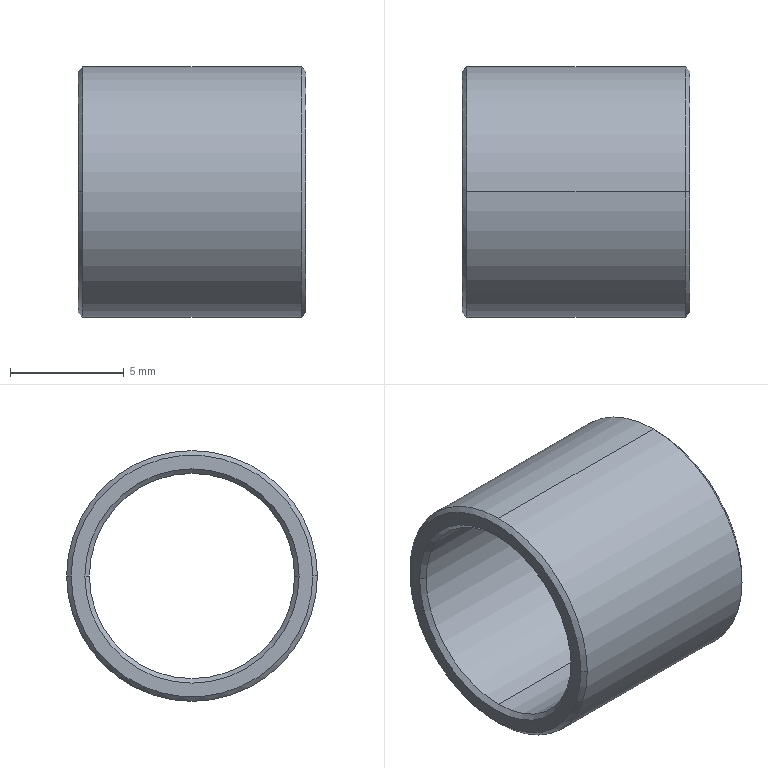Part | SolidWorks | features BaseBody 1 | 1 solid | 14 faces | box 10 x 11 x 11 mm | volume 311.646 mm3 | cone 8 | cylinder 4 | plane 2 | commonest cylinder face diameters 9 x2 11 x2
STEP:
#1=CARTESIAN_POINT('',(9.8,0.,5.5));
#2=VERTEX_POINT('',#1);
#3=CARTESIAN_POINT('',(9.8,0.,-5.5));
#4=VERTEX_POINT('',#3);
#5=CARTESIAN_POINT('',(9.8,0.,0.));
#6=DIRECTION('',(-1.,0.,0.));
#7=DIRECTION('',(0.,0.,1.));
#8=AXIS2_PLACEMENT_3D('',#5,#6,#7);
#9=CIRCLE('',#8,5.5);
#10=EDGE_CURVE('',#2,#4,#9,.T.);
#11=ORIENTED_EDGE('',*,*,#10,.T.);
#12=CARTESIAN_POINT('',(0.2,0.,-5.5));
#13=VERTEX_POINT('',#12);
#14=CARTESIAN_POINT('',(5.,0.,-5.5));
#15=DIRECTION('',(-1.,0.,0.));
#16=VECTOR('',#15,1000.);
#17=LINE('',#14,#16);
#18=EDGE_CURVE('',#4,#13,#17,.T.);
#19=ORIENTED_EDGE('',*,*,#18,.T.);
#20=CARTESIAN_POINT('',(0.2,5.5,0.));
#21=VERTEX_POINT('',#20);
#22=CARTESIAN_POINT('',(0.2,0.,0.));
#23=DIRECTION('',(1.,0.,0.));
#24=DIRECTION('',(0.,0.,1.));
#25=AXIS2_PLACEMENT_3D('',#22,#23,#24);
#26=CIRCLE('',#25,5.5);
#27=EDGE_CURVE('',#13,#21,#26,.T.);
#28=ORIENTED_EDGE('',*,*,#27,.T.);
#29=CARTESIAN_POINT('',(0.2,0.,5.5));
#30=VERTEX_POINT('',#29);
#31=CARTESIAN_POINT('',(0.2,0.,0.));
#32=DIRECTION('',(1.,0.,0.));
#33=DIRECTION('',(0.,0.,1.));
#34=AXIS2_PLACEMENT_3D('',#31,#32,#33);
#35=CIRCLE('',#34,5.5);
#36=EDGE_CURVE('',#21,#30,#35,.T.);
#37=ORIENTED_EDGE('',*,*,#36,.T.);
#38=CARTESIAN_POINT('',(5.,0.,5.5));
#39=DIRECTION('',(-1.,0.,0.));
#40=VECTOR('',#39,1000.);
#41=LINE('',#38,#40);
#42=EDGE_CURVE('',#2,#30,#41,.T.);
#43=ORIENTED_EDGE('',*,*,#42,.F.);
#44=EDGE_LOOP('',(#11,#19,#28,#37,#43));
#45=FACE_OUTER_BOUND('',#44,.T.);
#46=CARTESIAN_POINT('',(5.,0.,0.));
#47=DIRECTION('',(-1.,0.,0.));
#48=DIRECTION('',(0.,0.,1.));
#49=AXIS2_PLACEMENT_3D('',#46,#47,#48);
#50=CYLINDRICAL_SURFACE('',#49,5.5);
#51=ADVANCED_FACE('',(#45),#50,.T.);
#52=CARTESIAN_POINT('',(0.,5.3,0.));
#53=VERTEX_POINT('',#52);
#54=CARTESIAN_POINT('',(0.,-5.3,0.));
#55=VERTEX_POINT('',#54);
#56=CARTESIAN_POINT('',(0.,0.,0.));
#57=DIRECTION('',(1.,0.,0.));
#58=DIRECTION('',(0.,1.,0.));
#59=AXIS2_PLACEMENT_3D('',#56,#57,#58);
#60=CIRCLE('',#59,5.3);
#61=EDGE_CURVE('',#53,#55,#60,.T.);
#62=ORIENTED_EDGE('',*,*,#61,.T.);
#63=CARTESIAN_POINT('',(0.2,-5.5,0.));
#64=VERTEX_POINT('',#63);
#65=CARTESIAN_POINT('',(0.2,-5.5,0.));
#66=DIRECTION('',(0.7071,-0.7071,0.));
#67=VECTOR('',#66,1000.);
#68=LINE('',#65,#67);
#69=EDGE_CURVE('',#55,#64,#68,.T.);
#70=ORIENTED_EDGE('',*,*,#69,.T.);
#71=CARTESIAN_POINT('',(0.2,0.,0.));
#72=DIRECTION('',(1.,0.,0.));
#73=DIRECTION('',(0.,0.,1.));
#74=AXIS2_PLACEMENT_3D('',#71,#72,#73);
#75=CIRCLE('',#74,5.5);
#76=EDGE_CURVE('',#30,#64,#75,.T.);
#77=ORIENTED_EDGE('',*,*,#76,.F.);
#78=ORIENTED_EDGE('',*,*,#36,.F.);
#79=CARTESIAN_POINT('',(0.2,5.5,0.));
#80=DIRECTION('',(0.7071,0.7071,0.));
#81=VECTOR('',#80,1000.);
#82=LINE('',#79,#81);
#83=EDGE_CURVE('',#53,#21,#82,.T.);
#84=ORIENTED_EDGE('',*,*,#83,.F.);
#85=EDGE_LOOP('',(#62,#70,#77,#78,#84));
#86=FACE_OUTER_BOUND('',#85,.T.);
#87=CARTESIAN_POINT('',(0.2,0.,0.));
#88=DIRECTION('',(1.,0.,0.));
#89=DIRECTION('',(0.,1.,0.));
#90=AXIS2_PLACEMENT_3D('',#87,#88,#89);
#91=CONICAL_SURFACE('',#90,5.5,0.7854);
#92=ADVANCED_FACE('',(#86),#91,.T.);
#93=CARTESIAN_POINT('',(10.,0.,5.3));
#94=VERTEX_POINT('',#93);
#95=CARTESIAN_POINT('',(10.,0.,-5.3));
#96=VERTEX_POINT('',#95);
#97=CARTESIAN_POINT('',(10.,0.,0.));
#98=DIRECTION('',(-1.,0.,0.));
#99=DIRECTION('',(0.,0.,1.));
#100=AXIS2_PLACEMENT_3D('',#97,#98,#99);
#101=CIRCLE('',#100,5.3);
#102=EDGE_CURVE('',#94,#96,#101,.T.);
#103=ORIENTED_EDGE('',*,*,#102,.T.);
#104=CARTESIAN_POINT('',(9.8,0.,-5.5));
#105=DIRECTION('',(-0.7071,0.,-0.7071));
#106=VECTOR('',#105,1000.);
#107=LINE('',#104,#106);
#108=EDGE_CURVE('',#96,#4,#107,.T.);
#109=ORIENTED_EDGE('',*,*,#108,.T.);
#110=ORIENTED_EDGE('',*,*,#10,.F.);
#111=CARTESIAN_POINT('',(9.8,0.,5.5));
#112=DIRECTION('',(-0.7071,0.,0.7071));
#113=VECTOR('',#112,1000.);
#114=LINE('',#111,#113);
#115=EDGE_CURVE('',#94,#2,#114,.T.);
#116=ORIENTED_EDGE('',*,*,#115,.F.);
#117=EDGE_LOOP('',(#103,#109,#110,#116));
#118=FACE_OUTER_BOUND('',#117,.T.);
#119=CARTESIAN_POINT('',(9.8,0.,0.));
#120=DIRECTION('',(-1.,0.,0.));
#121=DIRECTION('',(0.,0.,1.));
#122=AXIS2_PLACEMENT_3D('',#119,#120,#121);
#123=CONICAL_SURFACE('',#122,5.5,0.7854);
#124=ADVANCED_FACE('',(#118),#123,.T.);
#125=CARTESIAN_POINT('',(0.2,4.5,0.));
#126=VERTEX_POINT('',#125);
#127=CARTESIAN_POINT('',(0.2,0.,-4.5));
#128=VERTEX_POINT('',#127);
#129=CARTESIAN_POINT('',(0.2,0.,0.));
#130=DIRECTION('',(-1.,0.,0.));
#131=DIRECTION('',(0.,-1.,0.));
#132=AXIS2_PLACEMENT_3D('',#129,#130,#131);
#133=CIRCLE('',#132,4.5);
#134=EDGE_CURVE('',#126,#128,#133,.T.);
#135=ORIENTED_EDGE('',*,*,#134,.F.);
#136=CARTESIAN_POINT('',(0.,4.7,0.));
#137=VERTEX_POINT('',#136);
#138=CARTESIAN_POINT('',(0.,4.7,0.));
#139=DIRECTION('',(-0.7071,0.7071,0.));
#140=VECTOR('',#139,1000.);
#141=LINE('',#138,#140);
#142=EDGE_CURVE('',#126,#137,#141,.T.);
#143=ORIENTED_EDGE('',*,*,#142,.T.);
#144=CARTESIAN_POINT('',(0.,-4.7,0.));
#145=VERTEX_POINT('',#144);
#146=CARTESIAN_POINT('',(0.,0.,0.));
#147=DIRECTION('',(1.,0.,0.));
#148=DIRECTION('',(0.,-1.,0.));
#149=AXIS2_PLACEMENT_3D('',#146,#147,#148);
#150=CIRCLE('',#149,4.7);
#151=EDGE_CURVE('',#145,#137,#150,.T.);
#152=ORIENTED_EDGE('',*,*,#151,.F.);
#153=CARTESIAN_POINT('',(0.2,-4.5,0.));
#154=VERTEX_POINT('',#153);
#155=CARTESIAN_POINT('',(0.,-4.7,0.));
#156=DIRECTION('',(-0.7071,-0.7071,0.));
#157=VECTOR('',#156,1000.);
#158=LINE('',#155,#157);
#159=EDGE_CURVE('',#154,#145,#158,.T.);
#160=ORIENTED_EDGE('',*,*,#159,.F.);
#161=CARTESIAN_POINT('',(0.2,0.,0.));
#162=DIRECTION('',(-1.,0.,0.));
#163=DIRECTION('',(0.,-1.,0.));
#164=AXIS2_PLACEMENT_3D('',#161,#162,#163);
#165=CIRCLE('',#164,4.5);
#166=EDGE_CURVE('',#128,#154,#165,.T.);
#167=ORIENTED_EDGE('',*,*,#166,.F.);
#168=EDGE_LOOP('',(#135,#143,#152,#160,#167));
#169=FACE_OUTER_BOUND('',#168,.T.);
#170=CARTESIAN_POINT('',(0.,0.,0.));
#171=DIRECTION('',(-1.,0.,0.));
#172=DIRECTION('',(0.,-1.,0.));
#173=AXIS2_PLACEMENT_3D('',#170,#171,#172);
#174=CONICAL_SURFACE('',#173,4.7,0.7854);
#175=ADVANCED_FACE('',(#169),#174,.F.);
#176=CARTESIAN_POINT('',(9.8,0.,4.5));
#177=VERTEX_POINT('',#176);
#178=CARTESIAN_POINT('',(9.8,0.,-4.5));
#179=VERTEX_POINT('',#178);
#180=CARTESIAN_POINT('',(9.8,0.,0.));
#181=DIRECTION('',(1.,0.,0.));
#182=DIRECTION('',(0.,-1.,0.));
#183=AXIS2_PLACEMENT_3D('',#180,#181,#182);
#184=CIRCLE('',#183,4.5);
#185=EDGE_CURVE('',#177,#179,#184,.T.);
#186=ORIENTED_EDGE('',*,*,#185,.F.);
#187=CARTESIAN_POINT('',(10.,0.,4.7));
#188=VERTEX_POINT('',#187);
#189=CARTESIAN_POINT('',(10.,0.,4.7));
#190=DIRECTION('',(0.7071,0.,0.7071));
#191=VECTOR('',#190,1000.);
#192=LINE('',#189,#191);
#193=EDGE_CURVE('',#177,#188,#192,.T.);
#194=ORIENTED_EDGE('',*,*,#193,.T.);
#195=CARTESIAN_POINT('',(10.,0.,-4.7));
#196=VERTEX_POINT('',#195);
#197=CARTESIAN_POINT('',(10.,0.,0.));
#198=DIRECTION('',(-1.,0.,0.));
#199=DIRECTION('',(0.,0.,-1.));
#200=AXIS2_PLACEMENT_3D('',#197,#198,#199);
#201=CIRCLE('',#200,4.7);
#202=EDGE_CURVE('',#196,#188,#201,.T.);
#203=ORIENTED_EDGE('',*,*,#202,.F.);
#204=CARTESIAN_POINT('',(10.,0.,-4.7));
#205=DIRECTION('',(0.7071,0.,-0.7071));
#206=VECTOR('',#205,1000.);
#207=LINE('',#204,#206);
#208=EDGE_CURVE('',#179,#196,#207,.T.);
#209=ORIENTED_EDGE('',*,*,#208,.F.);
#210=EDGE_LOOP('',(#186,#194,#203,#209));
#211=FACE_OUTER_BOUND('',#210,.T.);
#212=CARTESIAN_POINT('',(10.,0.,0.));
#213=DIRECTION('',(1.,0.,0.));
#214=DIRECTION('',(0.,0.,-1.));
#215=AXIS2_PLACEMENT_3D('',#212,#213,#214);
#216=CONICAL_SURFACE('',#215,4.7,0.7854);
#217=ADVANCED_FACE('',(#211),#216,.F.);
#218=ORIENTED_EDGE('',*,*,#185,.T.);
#219=CARTESIAN_POINT('',(5.,0.,-4.5));
#220=DIRECTION('',(-1.,0.,0.));
#221=VECTOR('',#220,1000.);
#222=LINE('',#219,#221);
#223=EDGE_CURVE('',#179,#128,#222,.T.);
#224=ORIENTED_EDGE('',*,*,#223,.T.);
#225=ORIENTED_EDGE('',*,*,#166,.T.);
#226=CARTESIAN_POINT('',(0.2,0.,4.5));
#227=VERTEX_POINT('',#226);
#228=CARTESIAN_POINT('',(0.2,0.,0.));
#229=DIRECTION('',(-1.,0.,0.));
#230=DIRECTION('',(0.,-1.,0.));
#231=AXIS2_PLACEMENT_3D('',#228,#229,#230);
#232=CIRCLE('',#231,4.5);
#233=EDGE_CURVE('',#154,#227,#232,.T.);
#234=ORIENTED_EDGE('',*,*,#233,.T.);
#235=CARTESIAN_POINT('',(5.,0.,4.5));
#236=DIRECTION('',(-1.,0.,0.));
#237=VECTOR('',#236,1000.);
#238=LINE('',#235,#237);
#239=EDGE_CURVE('',#177,#227,#238,.T.);
#240=ORIENTED_EDGE('',*,*,#239,.F.);
#241=EDGE_LOOP('',(#218,#224,#225,#234,#240));
#242=FACE_OUTER_BOUND('',#241,.T.);
#243=CARTESIAN_POINT('',(5.,0.,0.));
#244=DIRECTION('',(-1.,0.,0.));
#245=DIRECTION('',(0.,0.,1.));
#246=AXIS2_PLACEMENT_3D('',#243,#244,#245);
#247=CYLINDRICAL_SURFACE('',#246,4.5);
#248=ADVANCED_FACE('',(#242),#247,.F.);
#249=ORIENTED_EDGE('',*,*,#18,.F.);
#250=CARTESIAN_POINT('',(9.8,0.,0.));
#251=DIRECTION('',(-1.,0.,0.));
#252=DIRECTION('',(0.,0.,1.));
#253=AXIS2_PLACEMENT_3D('',#250,#251,#252);
#254=CIRCLE('',#253,5.5);
#255=EDGE_CURVE('',#4,#2,#254,.T.);
#256=ORIENTED_EDGE('',*,*,#255,.T.);
#257=ORIENTED_EDGE('',*,*,#42,.T.);
#258=ORIENTED_EDGE('',*,*,#76,.T.);
#259=CARTESIAN_POINT('',(0.2,0.,0.));
#260=DIRECTION('',(1.,0.,0.));
#261=DIRECTION('',(0.,0.,1.));
#262=AXIS2_PLACEMENT_3D('',#259,#260,#261);
#263=CIRCLE('',#262,5.5);
#264=EDGE_CURVE('',#64,#13,#263,.T.);
#265=ORIENTED_EDGE('',*,*,#264,.T.);
#266=EDGE_LOOP('',(#249,#256,#257,#258,#265));
#267=FACE_OUTER_BOUND('',#266,.T.);
#268=CARTESIAN_POINT('',(5.,0.,0.));
#269=DIRECTION('',(-1.,0.,0.));
#270=DIRECTION('',(0.,0.,1.));
#271=AXIS2_PLACEMENT_3D('',#268,#269,#270);
#272=CYLINDRICAL_SURFACE('',#271,5.5);
#273=ADVANCED_FACE('',(#267),#272,.T.);
#274=ORIENTED_EDGE('',*,*,#69,.F.);
#275=CARTESIAN_POINT('',(0.,0.,0.));
#276=DIRECTION('',(1.,0.,0.));
#277=DIRECTION('',(0.,1.,0.));
#278=AXIS2_PLACEMENT_3D('',#275,#276,#277);
#279=CIRCLE('',#278,5.3);
#280=EDGE_CURVE('',#55,#53,#279,.T.);
#281=ORIENTED_EDGE('',*,*,#280,.T.);
#282=ORIENTED_EDGE('',*,*,#83,.T.);
#283=ORIENTED_EDGE('',*,*,#27,.F.);
#284=ORIENTED_EDGE('',*,*,#264,.F.);
#285=EDGE_LOOP('',(#274,#281,#282,#283,#284));
#286=FACE_OUTER_BOUND('',#285,.T.);
#287=CARTESIAN_POINT('',(0.2,0.,0.));
#288=DIRECTION('',(1.,0.,0.));
#289=DIRECTION('',(0.,1.,0.));
#290=AXIS2_PLACEMENT_3D('',#287,#288,#289);
#291=CONICAL_SURFACE('',#290,5.5,0.7854);
#292=ADVANCED_FACE('',(#286),#291,.T.);
#293=ORIENTED_EDGE('',*,*,#108,.F.);
#294=CARTESIAN_POINT('',(10.,0.,0.));
#295=DIRECTION('',(-1.,0.,0.));
#296=DIRECTION('',(0.,0.,1.));
#297=AXIS2_PLACEMENT_3D('',#294,#295,#296);
#298=CIRCLE('',#297,5.3);
#299=EDGE_CURVE('',#96,#94,#298,.T.);
#300=ORIENTED_EDGE('',*,*,#299,.T.);
#301=ORIENTED_EDGE('',*,*,#115,.T.);
#302=ORIENTED_EDGE('',*,*,#255,.F.);
#303=EDGE_LOOP('',(#293,#300,#301,#302));
#304=FACE_OUTER_BOUND('',#303,.T.);
#305=CARTESIAN_POINT('',(9.8,0.,0.));
#306=DIRECTION('',(-1.,0.,0.));
#307=DIRECTION('',(0.,0.,1.));
#308=AXIS2_PLACEMENT_3D('',#305,#306,#307);
#309=CONICAL_SURFACE('',#308,5.5,0.7854);
#310=ADVANCED_FACE('',(#304),#309,.T.);
#311=ORIENTED_EDGE('',*,*,#61,.F.);
#312=ORIENTED_EDGE('',*,*,#280,.F.);
#313=EDGE_LOOP('',(#311,#312));
#314=FACE_OUTER_BOUND('',#313,.T.);
#315=ORIENTED_EDGE('',*,*,#151,.T.);
#316=CARTESIAN_POINT('',(0.,0.,0.));
#317=DIRECTION('',(1.,0.,0.));
#318=DIRECTION('',(0.,-1.,0.));
#319=AXIS2_PLACEMENT_3D('',#316,#317,#318);
#320=CIRCLE('',#319,4.7);
#321=EDGE_CURVE('',#137,#145,#320,.T.);
#322=ORIENTED_EDGE('',*,*,#321,.T.);
#323=EDGE_LOOP('',(#315,#322));
#324=FACE_BOUND('',#323,.T.);
#325=CARTESIAN_POINT('',(0.,-2.75,0.));
#326=DIRECTION('',(-1.,0.,0.));
#327=DIRECTION('',(0.,0.,1.));
#328=AXIS2_PLACEMENT_3D('',#325,#326,#327);
#329=PLANE('',#328);
#330=ADVANCED_FACE('',(#314,#324),#329,.T.);
#331=ORIENTED_EDGE('',*,*,#202,.T.);
#332=CARTESIAN_POINT('',(10.,0.,0.));
#333=DIRECTION('',(-1.,0.,0.));
#334=DIRECTION('',(0.,0.,-1.));
#335=AXIS2_PLACEMENT_3D('',#332,#333,#334);
#336=CIRCLE('',#335,4.7);
#337=EDGE_CURVE('',#188,#196,#336,.T.);
#338=ORIENTED_EDGE('',*,*,#337,.T.);
#339=EDGE_LOOP('',(#331,#338));
#340=FACE_BOUND('',#339,.T.);
#341=ORIENTED_EDGE('',*,*,#102,.F.);
#342=ORIENTED_EDGE('',*,*,#299,.F.);
#343=EDGE_LOOP('',(#341,#342));
#344=FACE_OUTER_BOUND('',#343,.T.);
#345=CARTESIAN_POINT('',(10.,-2.75,0.));
#346=DIRECTION('',(1.,0.,0.));
#347=DIRECTION('',(0.,0.,-1.));
#348=AXIS2_PLACEMENT_3D('',#345,#346,#347);
#349=PLANE('',#348);
#350=ADVANCED_FACE('',(#340,#344),#349,.T.);
#351=ORIENTED_EDGE('',*,*,#142,.F.);
#352=CARTESIAN_POINT('',(0.2,0.,0.));
#353=DIRECTION('',(-1.,0.,0.));
#354=DIRECTION('',(0.,-1.,0.));
#355=AXIS2_PLACEMENT_3D('',#352,#353,#354);
#356=CIRCLE('',#355,4.5);
#357=EDGE_CURVE('',#227,#126,#356,.T.);
#358=ORIENTED_EDGE('',*,*,#357,.F.);
#359=ORIENTED_EDGE('',*,*,#233,.F.);
#360=ORIENTED_EDGE('',*,*,#159,.T.);
#361=ORIENTED_EDGE('',*,*,#321,.F.);
#362=EDGE_LOOP('',(#351,#358,#359,#360,#361));
#363=FACE_OUTER_BOUND('',#362,.T.);
#364=CARTESIAN_POINT('',(0.,0.,0.));
#365=DIRECTION('',(-1.,0.,0.));
#366=DIRECTION('',(0.,-1.,0.));
#367=AXIS2_PLACEMENT_3D('',#364,#365,#366);
#368=CONICAL_SURFACE('',#367,4.7,0.7854);
#369=ADVANCED_FACE('',(#363),#368,.F.);
#370=ORIENTED_EDGE('',*,*,#193,.F.);
#371=CARTESIAN_POINT('',(9.8,0.,0.));
#372=DIRECTION('',(1.,0.,0.));
#373=DIRECTION('',(0.,-1.,0.));
#374=AXIS2_PLACEMENT_3D('',#371,#372,#373);
#375=CIRCLE('',#374,4.5);
#376=EDGE_CURVE('',#179,#177,#375,.T.);
#377=ORIENTED_EDGE('',*,*,#376,.F.);
#378=ORIENTED_EDGE('',*,*,#208,.T.);
#379=ORIENTED_EDGE('',*,*,#337,.F.);
#380=EDGE_LOOP('',(#370,#377,#378,#379));
#381=FACE_OUTER_BOUND('',#380,.T.);
#382=CARTESIAN_POINT('',(10.,0.,0.));
#383=DIRECTION('',(1.,0.,0.));
#384=DIRECTION('',(0.,0.,-1.));
#385=AXIS2_PLACEMENT_3D('',#382,#383,#384);
#386=CONICAL_SURFACE('',#385,4.7,0.7854);
#387=ADVANCED_FACE('',(#381),#386,.F.);
#388=ORIENTED_EDGE('',*,*,#223,.F.);
#389=ORIENTED_EDGE('',*,*,#376,.T.);
#390=ORIENTED_EDGE('',*,*,#239,.T.);
#391=ORIENTED_EDGE('',*,*,#357,.T.);
#392=ORIENTED_EDGE('',*,*,#134,.T.);
#393=EDGE_LOOP('',(#388,#389,#390,#391,#392));
#394=FACE_OUTER_BOUND('',#393,.T.);
#395=CARTESIAN_POINT('',(5.,0.,0.));
#396=DIRECTION('',(-1.,0.,0.));
#397=DIRECTION('',(0.,0.,1.));
#398=AXIS2_PLACEMENT_3D('',#395,#396,#397);
#399=CYLINDRICAL_SURFACE('',#398,4.5);
#400=ADVANCED_FACE('',(#394),#399,.F.);
#401=CLOSED_SHELL('',(#51,#92,#124,#175,#217,#248,#273,#292,#310,#330,#350,#369,#387,#400));
#402=MANIFOLD_SOLID_BREP('',#401);
#403=CARTESIAN_POINT('',(0.,0.,0.));
#404=DIRECTION('',(0.,0.,1.));
#405=DIRECTION('',(1.,0.,0.));
#406=AXIS2_PLACEMENT_3D('',#403,#404,#405);
#407=(LENGTH_UNIT()NAMED_UNIT(*)SI_UNIT(.MILLI.,.METRE.));
#408=UNCERTAINTY_MEASURE_WITH_UNIT(LENGTH_MEASURE(0.00001),#407,'','');
#409=(NAMED_UNIT(*)PLANE_ANGLE_UNIT()SI_UNIT($,.RADIAN.));
#410=(NAMED_UNIT(*)SI_UNIT($,.STERADIAN.)SOLID_ANGLE_UNIT());
#411=(GEOMETRIC_REPRESENTATION_CONTEXT(3)GLOBAL_UNCERTAINTY_ASSIGNED_CONTEXT((#408))GLOBAL_UNIT_ASSIGNED_CONTEXT((#407,#409,#410))REPRESENTATION_CONTEXT('',''));
#412=ADVANCED_BREP_SHAPE_REPRESENTATION('',(#402,#406),#411);